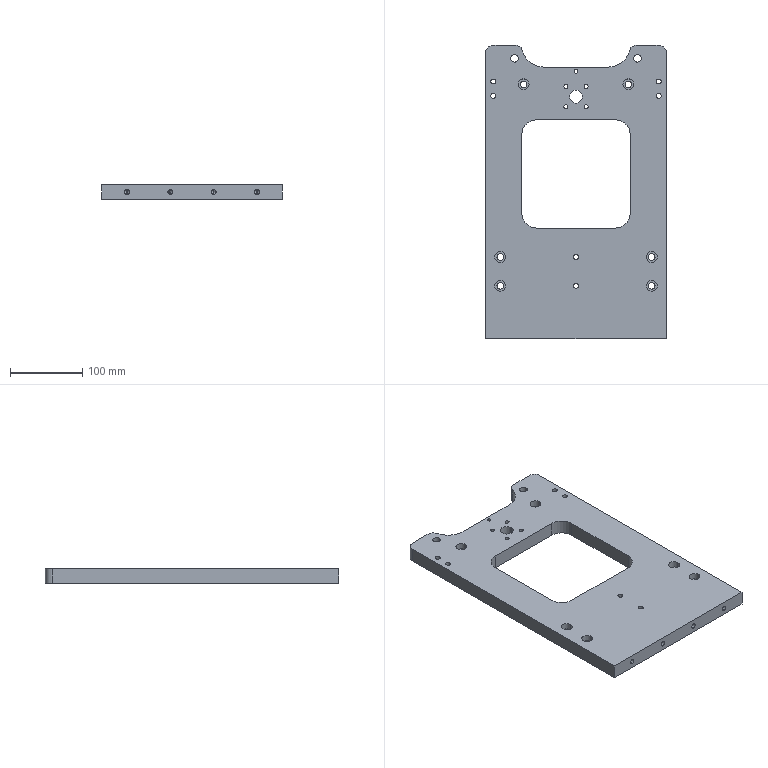Part | 1 solid | 108 faces | box 250 x 406 x 20 mm | volume 1469974 mm3 | cylinder 78 | plane 22 | cone 8 | commonest cylinder face diameters 6.8 x20 9 x12 15 x12 5.5 x8 10 x8 10.5 x4